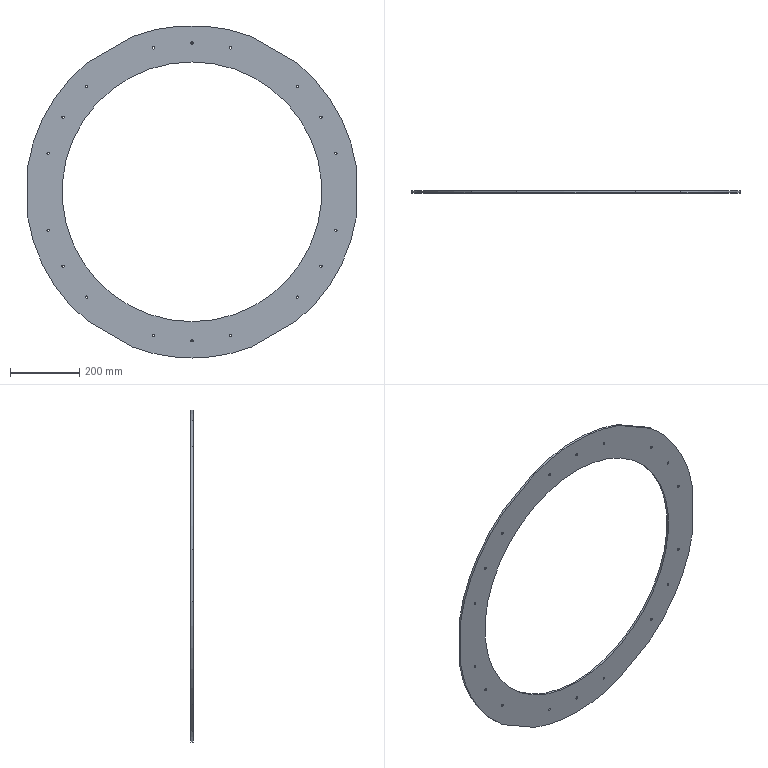Part | SolidWorks | features CirPattern 1, Extrusion 1, HoleWzd 1, ICE 1 | 1 solid | 53 faces | box 948 x 6 x 960 mm | volume 1666480 mm3 | cylinder 45 | plane 8 | commonest cylinder face diameters 6.8 x36 960 x7 750 x2